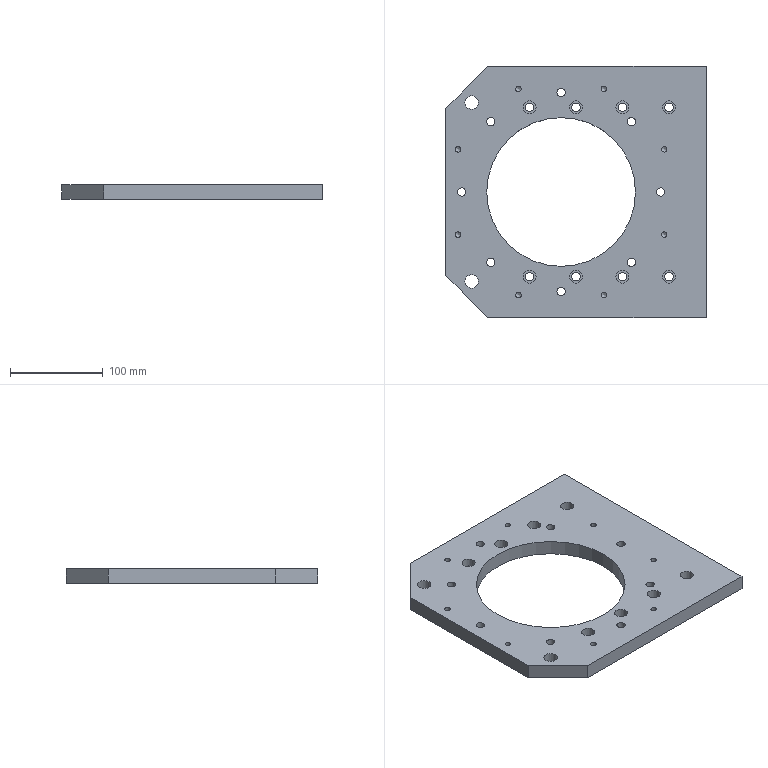Part | 1 solid | 83 faces | box 280 x 270 x 16 mm | volume 815522 mm3 | cylinder 47 | plane 24 | cone 12 | commonest cylinder face diameters 9 x16 14 x16 6 x8 6.8 x4 14.5 x2 160 x1